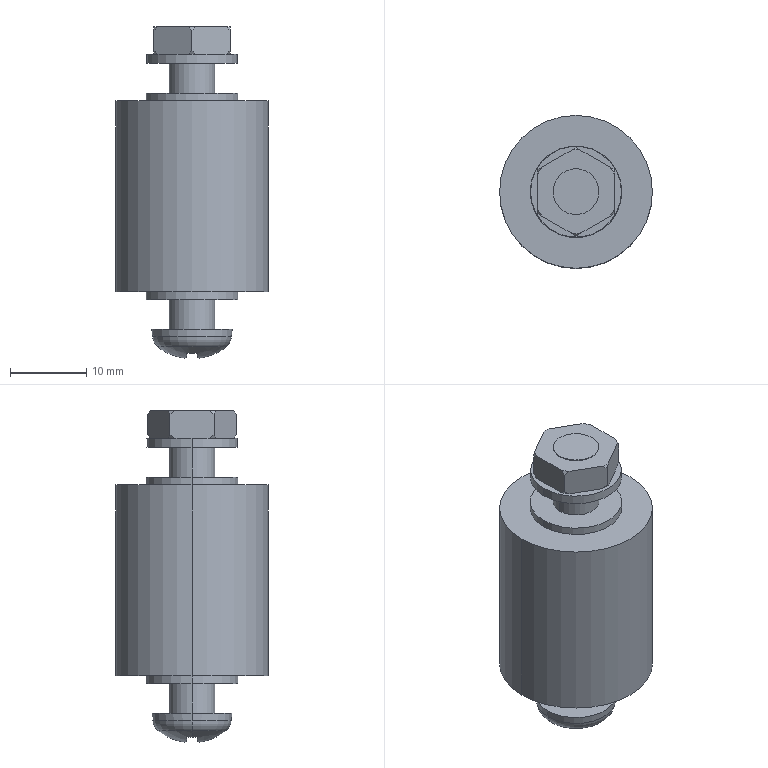Part | STEP file | Mirror ROLLER-2_0829_041_CRONWB29 | 1 solid | 64 faces | box 20 x 20 x 43.458 mm | volume 8966 mm3 | plane 28 | cylinder 18 | cone 14 | sphere 2 | torus 2 | commonest cylinder face diameters 6 x6 2 x4 12 x4 11.9 x2 20 x2